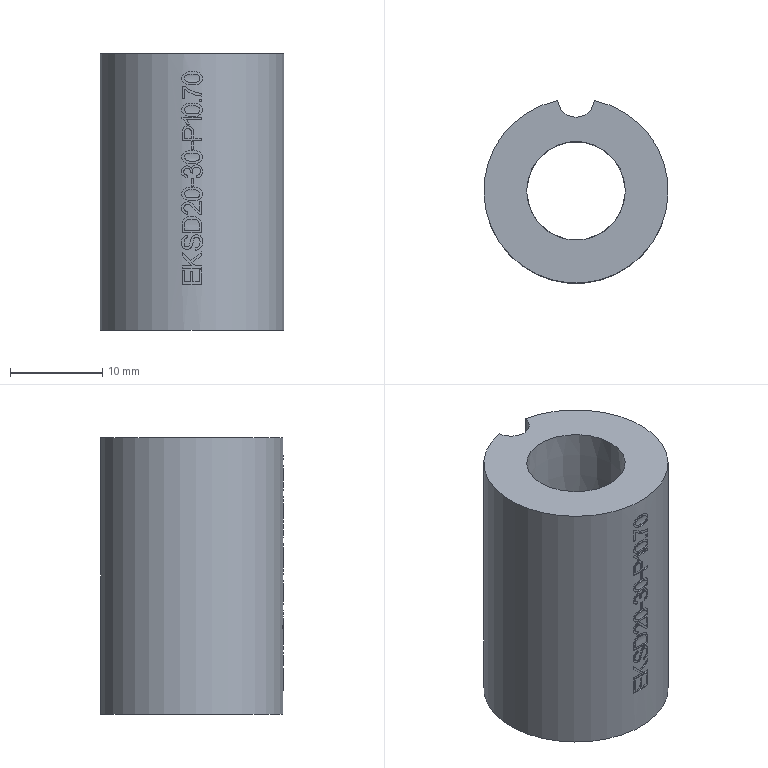Part | NX | features EKSD20-30-P10.70_2 2 | 1 solid | 207 faces | box 20 x 19.801 x 30 mm | volume 5776 mm3 | plane 116 | cylinder 90 | cone 1 | commonest cylinder face diameters 19.8 x16 20 x7 0.921 x4 1.098 x4 1.102 x4 1.115 x4